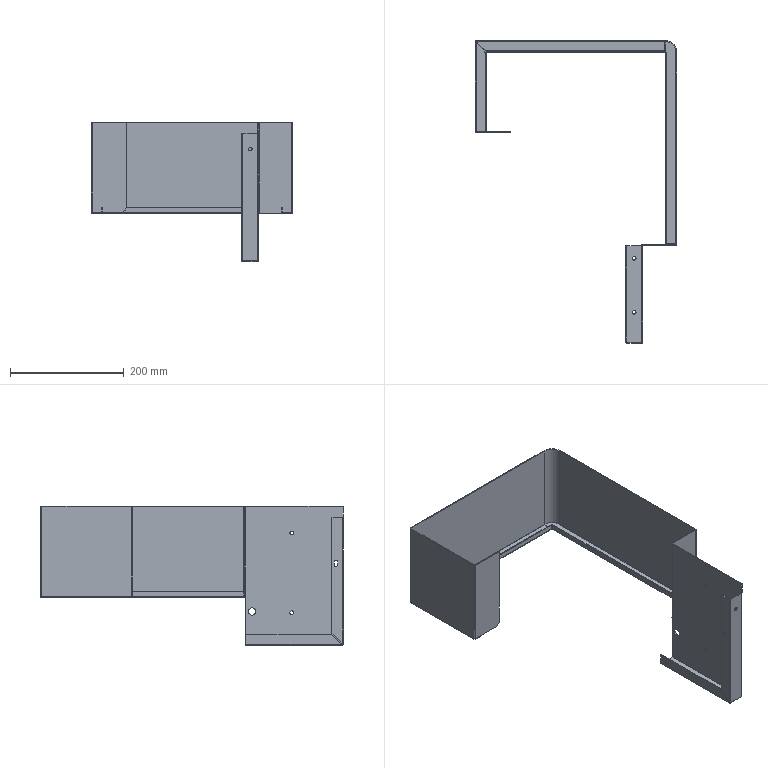Part | SolidWorks | features ICE 14, EdgeFlange 4, SMMiteredFlange 3, SMBaseFlange 2, Cut 1, Fillet 1, FlatPattern 1, LPattern 1, SheetMetal 1 | 1 solid | 181 faces | box 355 x 533 x 245 mm | volume 356884 mm3 | plane 127 | cylinder 48 | spline 6 | commonest cylinder face diameters 1 x14 4 x14 6.4 x10 13 x4 6 x2 20 x1